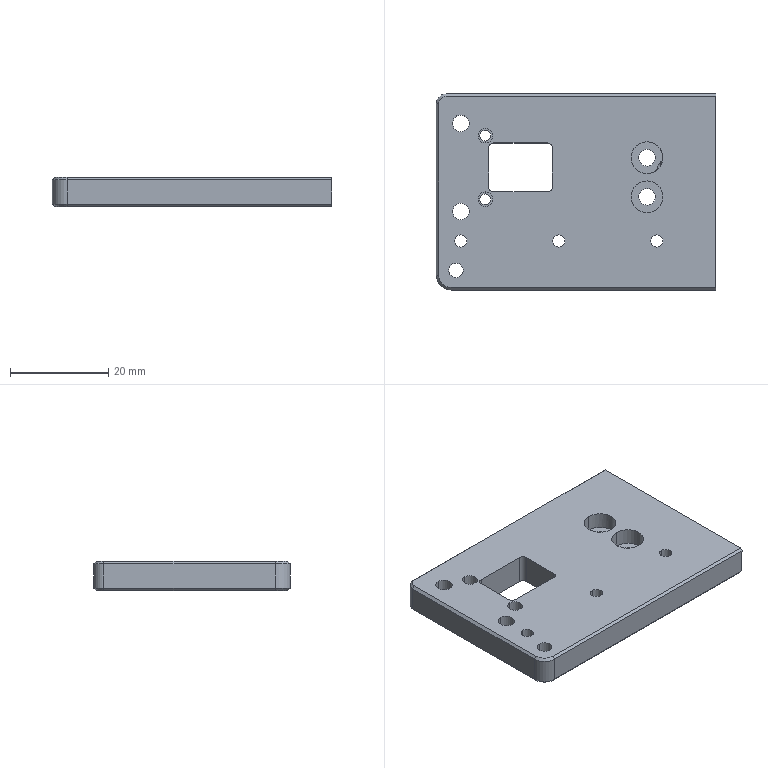Part | 1 solid | 89 faces | box 57 x 40 x 6 mm | volume 11770 mm3 | cylinder 48 | plane 26 | cone 15 | commonest cylinder face diameters 2.5 x12 3 x10 3.4 x8 6.5 x8 2 x4 2.2 x4